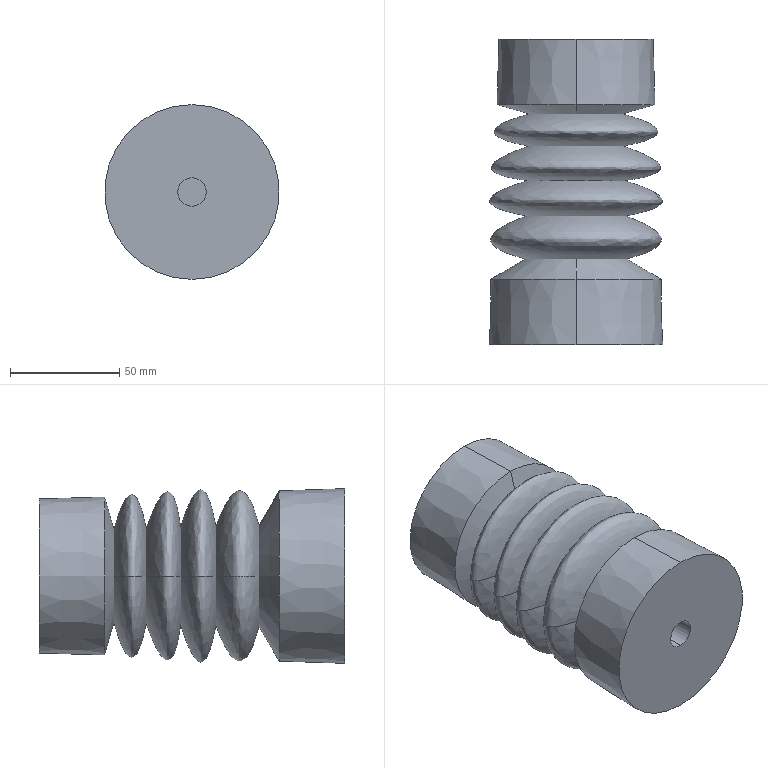Part | STEP file | High voltage insulator | 1 solid | 30 faces | box 80 x 140 x 80 mm | volume 533593 mm3 | spline 8 | cylinder 8 | cone 8 | plane 6 | commonest cylinder face diameters 8 x4 12 x2 13 x2